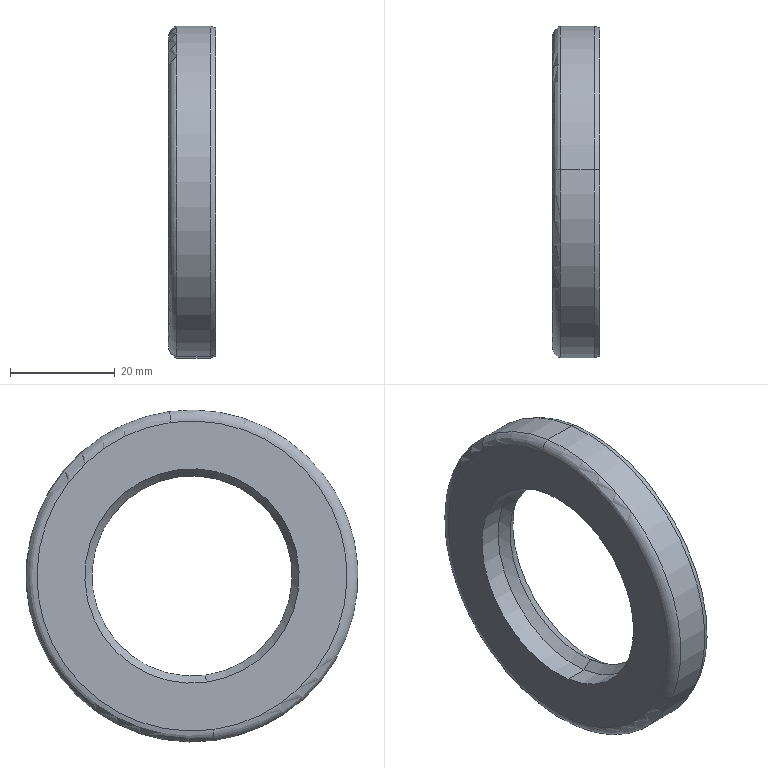Part | NX | features BREP 1 | 1 solid | 32 faces | box 9 x 63.5 x 63.5 mm | volume 6272 mm3 | torus 10 | cylinder 10 | cone 8 | plane 4 | commonest cylinder face diameters 45.17 x4 41 x2 61.3 x2 63.5 x2
STEP:
#1=CARTESIAN_POINT('',(-548.52,3.047,22.378));
#2=VERTEX_POINT('',#1);
#3=CARTESIAN_POINT('',(-548.52,-3.047,-22.378));
#4=VERTEX_POINT('',#3);
#5=CARTESIAN_POINT('',(-548.52,0.,0.));
#6=DIRECTION('',(-1.,0.,0.));
#7=DIRECTION('',(0.,0.1349,0.9909));
#8=AXIS2_PLACEMENT_3D('',#5,#6,#7);
#9=CIRCLE('',#8,22.585);
#10=EDGE_CURVE('',#2,#4,#9,.T.);
#11=ORIENTED_EDGE('',*,*,#10,.T.);
#12=CARTESIAN_POINT('',(-551.12,-3.047,-22.378));
#13=VERTEX_POINT('',#12);
#14=CARTESIAN_POINT('',(-549.82,-3.047,-22.378));
#15=DIRECTION('',(0.,0.9909,-0.1349));
#16=DIRECTION('',(0.,0.1349,0.9909));
#17=AXIS2_PLACEMENT_3D('',#14,#15,#16);
#18=CIRCLE('',#17,1.3);
#19=EDGE_CURVE('',#4,#13,#18,.T.);
#20=ORIENTED_EDGE('',*,*,#19,.T.);
#21=CARTESIAN_POINT('',(-551.12,3.047,22.378));
#22=VERTEX_POINT('',#21);
#23=CARTESIAN_POINT('',(-551.12,0.,0.));
#24=DIRECTION('',(1.,0.,0.));
#25=DIRECTION('',(0.,-0.1349,-0.9909));
#26=AXIS2_PLACEMENT_3D('',#23,#24,#25);
#27=CIRCLE('',#26,22.585);
#28=EDGE_CURVE('',#13,#22,#27,.T.);
#29=ORIENTED_EDGE('',*,*,#28,.T.);
#30=CARTESIAN_POINT('',(-549.82,3.047,22.378));
#31=DIRECTION('',(0.,-0.9909,0.1349));
#32=DIRECTION('',(0.,-0.1349,-0.9909));
#33=AXIS2_PLACEMENT_3D('',#30,#31,#32);
#34=CIRCLE('',#33,1.3);
#35=EDGE_CURVE('',#2,#22,#34,.T.);
#36=ORIENTED_EDGE('',*,*,#35,.F.);
#37=EDGE_LOOP('',(#11,#20,#29,#36));
#38=FACE_BOUND('',#37,.T.);
#39=CARTESIAN_POINT('',(-549.82,0.,0.));
#40=DIRECTION('',(-1.,0.,0.));
#41=DIRECTION('',(0.,-0.1349,-0.9909));
#42=AXIS2_PLACEMENT_3D('',#39,#40,#41);
#43=TOROIDAL_SURFACE('',#42,22.585,1.3);
#44=ADVANCED_FACE('',(#38),#43,.T.);
#45=CARTESIAN_POINT('',(-548.02,4.284,31.46));
#46=VERTEX_POINT('',#45);
#47=CARTESIAN_POINT('',(-548.02,-4.284,-31.46));
#48=VERTEX_POINT('',#47);
#49=CARTESIAN_POINT('',(-548.02,0.,0.));
#50=DIRECTION('',(-1.,0.,0.));
#51=DIRECTION('',(0.,0.1349,0.9909));
#52=AXIS2_PLACEMENT_3D('',#49,#50,#51);
#53=CIRCLE('',#52,31.75);
#54=EDGE_CURVE('',#46,#48,#53,.T.);
#55=ORIENTED_EDGE('',*,*,#54,.T.);
#56=CARTESIAN_POINT('',(-554.476,-4.284,-31.46));
#57=VERTEX_POINT('',#56);
#58=CARTESIAN_POINT('',(-556.022,-4.284,-31.46));
#59=DIRECTION('',(-1.,0.,0.));
#60=VECTOR('',#59,1000.);
#61=LINE('',#58,#60);
#62=EDGE_CURVE('',#48,#57,#61,.T.);
#63=ORIENTED_EDGE('',*,*,#62,.T.);
#64=CARTESIAN_POINT('',(-554.476,4.284,31.46));
#65=VERTEX_POINT('',#64);
#66=CARTESIAN_POINT('',(-554.476,0.,0.));
#67=DIRECTION('',(-1.,0.,0.));
#68=DIRECTION('',(0.,0.1349,0.9909));
#69=AXIS2_PLACEMENT_3D('',#66,#67,#68);
#70=CIRCLE('',#69,31.75);
#71=EDGE_CURVE('',#65,#57,#70,.T.);
#72=ORIENTED_EDGE('',*,*,#71,.F.);
#73=CARTESIAN_POINT('',(-556.022,4.284,31.46));
#74=DIRECTION('',(-1.,0.,0.));
#75=VECTOR('',#74,1000.);
#76=LINE('',#73,#75);
#77=EDGE_CURVE('',#46,#65,#76,.T.);
#78=ORIENTED_EDGE('',*,*,#77,.F.);
#79=EDGE_LOOP('',(#55,#63,#72,#78));
#80=FACE_BOUND('',#79,.T.);
#81=CARTESIAN_POINT('',(-556.022,0.,0.));
#82=DIRECTION('',(-1.,0.,0.));
#83=DIRECTION('',(0.,-0.1349,-0.9909));
#84=AXIS2_PLACEMENT_3D('',#81,#82,#83);
#85=CYLINDRICAL_SURFACE('',#84,31.75);
#86=ADVANCED_FACE('',(#80),#85,.T.);
#87=CARTESIAN_POINT('',(-547.02,4.235,31.099));
#88=VERTEX_POINT('',#87);
#89=CARTESIAN_POINT('',(-547.02,-4.235,-31.099));
#90=VERTEX_POINT('',#89);
#91=CARTESIAN_POINT('',(-547.02,0.,0.));
#92=DIRECTION('',(-1.,0.,0.));
#93=DIRECTION('',(0.,0.1349,0.9909));
#94=AXIS2_PLACEMENT_3D('',#91,#92,#93);
#95=CIRCLE('',#94,31.386);
#96=EDGE_CURVE('',#88,#90,#95,.T.);
#97=ORIENTED_EDGE('',*,*,#96,.T.);
#98=CARTESIAN_POINT('',(-547.02,-4.235,-31.099));
#99=DIRECTION('',(-0.9397,-0.04615,-0.3389));
#100=VECTOR('',#99,1000.);
#101=LINE('',#98,#100);
#102=EDGE_CURVE('',#90,#48,#101,.T.);
#103=ORIENTED_EDGE('',*,*,#102,.T.);
#104=ORIENTED_EDGE('',*,*,#54,.F.);
#105=CARTESIAN_POINT('',(-547.02,4.235,31.099));
#106=DIRECTION('',(-0.9397,0.04615,0.3389));
#107=VECTOR('',#106,1000.);
#108=LINE('',#105,#107);
#109=EDGE_CURVE('',#88,#46,#108,.T.);
#110=ORIENTED_EDGE('',*,*,#109,.F.);
#111=EDGE_LOOP('',(#97,#103,#104,#110));
#112=FACE_BOUND('',#111,.T.);
#113=CARTESIAN_POINT('',(-547.02,0.,0.));
#114=DIRECTION('',(-1.,0.,0.));
#115=DIRECTION('',(0.,-0.1349,-0.9909));
#116=AXIS2_PLACEMENT_3D('',#113,#114,#115);
#117=CONICAL_SURFACE('',#116,31.386,0.3491);
#118=ADVANCED_FACE('',(#112),#117,.T.);
#119=CARTESIAN_POINT('',(-547.02,-4.136,-30.37));
#120=VERTEX_POINT('',#119);
#121=CARTESIAN_POINT('',(-547.02,4.136,30.37));
#122=VERTEX_POINT('',#121);
#123=CARTESIAN_POINT('',(-547.02,0.,0.));
#124=DIRECTION('',(-1.,0.,0.));
#125=DIRECTION('',(0.,0.1349,0.9909));
#126=AXIS2_PLACEMENT_3D('',#123,#124,#125);
#127=CIRCLE('',#126,30.65);
#128=EDGE_CURVE('',#120,#122,#127,.T.);
#129=ORIENTED_EDGE('',*,*,#128,.F.);
#130=CARTESIAN_POINT('',(-553.82,-4.136,-30.37));
#131=VERTEX_POINT('',#130);
#132=CARTESIAN_POINT('',(-556.022,-4.136,-30.37));
#133=DIRECTION('',(-1.,0.,0.));
#134=VECTOR('',#133,1000.);
#135=LINE('',#132,#134);
#136=EDGE_CURVE('',#120,#131,#135,.T.);
#137=ORIENTED_EDGE('',*,*,#136,.T.);
#138=CARTESIAN_POINT('',(-553.82,4.136,30.37));
#139=VERTEX_POINT('',#138);
#140=CARTESIAN_POINT('',(-553.82,0.,0.));
#141=DIRECTION('',(-1.,0.,0.));
#142=DIRECTION('',(0.,0.1349,0.9909));
#143=AXIS2_PLACEMENT_3D('',#140,#141,#142);
#144=CIRCLE('',#143,30.65);
#145=EDGE_CURVE('',#131,#139,#144,.T.);
#146=ORIENTED_EDGE('',*,*,#145,.T.);
#147=CARTESIAN_POINT('',(-556.022,4.136,30.37));
#148=DIRECTION('',(-1.,0.,0.));
#149=VECTOR('',#148,1000.);
#150=LINE('',#147,#149);
#151=EDGE_CURVE('',#122,#139,#150,.T.);
#152=ORIENTED_EDGE('',*,*,#151,.F.);
#153=EDGE_LOOP('',(#129,#137,#146,#152));
#154=FACE_BOUND('',#153,.T.);
#155=CARTESIAN_POINT('',(-556.022,0.,0.));
#156=DIRECTION('',(-1.,0.,0.));
#157=DIRECTION('',(0.,-0.1349,-0.9909));
#158=AXIS2_PLACEMENT_3D('',#155,#156,#157);
#159=CYLINDRICAL_SURFACE('',#158,30.65);
#160=ADVANCED_FACE('',(#154),#159,.F.);
#161=ORIENTED_EDGE('',*,*,#145,.F.);
#162=CARTESIAN_POINT('',(-554.82,-4.001,-29.379));
#163=VERTEX_POINT('',#162);
#164=CARTESIAN_POINT('',(-553.82,-4.001,-29.379));
#165=DIRECTION('',(0.,0.9909,-0.1349));
#166=DIRECTION('',(0.,0.1349,0.9909));
#167=AXIS2_PLACEMENT_3D('',#164,#165,#166);
#168=CIRCLE('',#167,1.);
#169=EDGE_CURVE('',#131,#163,#168,.T.);
#170=ORIENTED_EDGE('',*,*,#169,.T.);
#171=CARTESIAN_POINT('',(-554.82,4.001,29.379));
#172=VERTEX_POINT('',#171);
#173=CARTESIAN_POINT('',(-554.82,0.,0.));
#174=DIRECTION('',(-1.,0.,0.));
#175=DIRECTION('',(0.,0.1349,0.9909));
#176=AXIS2_PLACEMENT_3D('',#173,#174,#175);
#177=CIRCLE('',#176,29.65);
#178=EDGE_CURVE('',#163,#172,#177,.T.);
#179=ORIENTED_EDGE('',*,*,#178,.T.);
#180=CARTESIAN_POINT('',(-553.82,4.001,29.379));
#181=DIRECTION('',(0.,-0.9909,0.1349));
#182=DIRECTION('',(0.,-0.1349,-0.9909));
#183=AXIS2_PLACEMENT_3D('',#180,#181,#182);
#184=CIRCLE('',#183,1.);
#185=EDGE_CURVE('',#139,#172,#184,.T.);
#186=ORIENTED_EDGE('',*,*,#185,.F.);
#187=EDGE_LOOP('',(#161,#170,#179,#186));
#188=FACE_BOUND('',#187,.T.);
#189=CARTESIAN_POINT('',(-553.82,0.,0.));
#190=DIRECTION('',(-1.,0.,0.));
#191=DIRECTION('',(0.,-0.1349,-0.9909));
#192=AXIS2_PLACEMENT_3D('',#189,#190,#191);
#193=TOROIDAL_SURFACE('',#192,29.65,1.);
#194=ADVANCED_FACE('',(#188),#193,.F.);
#195=ORIENTED_EDGE('',*,*,#71,.T.);
#196=CARTESIAN_POINT('',(-556.02,-4.001,-29.379));
#197=VERTEX_POINT('',#196);
#198=CARTESIAN_POINT('',(-553.82,-4.001,-29.379));
#199=DIRECTION('',(0.,0.9909,-0.1349));
#200=DIRECTION('',(0.,0.1349,0.9909));
#201=AXIS2_PLACEMENT_3D('',#198,#199,#200);
#202=CIRCLE('',#201,2.2);
#203=EDGE_CURVE('',#57,#197,#202,.T.);
#204=ORIENTED_EDGE('',*,*,#203,.T.);
#205=CARTESIAN_POINT('',(-556.02,4.001,29.379));
#206=VERTEX_POINT('',#205);
#207=CARTESIAN_POINT('',(-556.02,0.,0.));
#208=DIRECTION('',(-1.,0.,0.));
#209=DIRECTION('',(0.,0.1349,0.9909));
#210=AXIS2_PLACEMENT_3D('',#207,#208,#209);
#211=CIRCLE('',#210,29.65);
#212=EDGE_CURVE('',#206,#197,#211,.T.);
#213=ORIENTED_EDGE('',*,*,#212,.F.);
#214=CARTESIAN_POINT('',(-553.82,4.001,29.379));
#215=DIRECTION('',(0.,-0.9909,0.1349));
#216=DIRECTION('',(0.,-0.1349,-0.9909));
#217=AXIS2_PLACEMENT_3D('',#214,#215,#216);
#218=CIRCLE('',#217,2.2);
#219=EDGE_CURVE('',#65,#206,#218,.T.);
#220=ORIENTED_EDGE('',*,*,#219,.F.);
#221=EDGE_LOOP('',(#195,#204,#213,#220));
#222=FACE_BOUND('',#221,.T.);
#223=CARTESIAN_POINT('',(-553.82,0.,0.));
#224=DIRECTION('',(-1.,0.,0.));
#225=DIRECTION('',(0.,-0.1349,-0.9909));
#226=AXIS2_PLACEMENT_3D('',#223,#224,#225);
#227=TOROIDAL_SURFACE('',#226,29.65,2.2);
#228=ADVANCED_FACE('',(#222),#227,.T.);
#229=ORIENTED_EDGE('',*,*,#28,.F.);
#230=CARTESIAN_POINT('',(-554.,-3.047,-22.378));
#231=VERTEX_POINT('',#230);
#232=CARTESIAN_POINT('',(-556.022,-3.047,-22.378));
#233=DIRECTION('',(-1.,0.,0.));
#234=VECTOR('',#233,1000.);
#235=LINE('',#232,#234);
#236=EDGE_CURVE('',#13,#231,#235,.T.);
#237=ORIENTED_EDGE('',*,*,#236,.T.);
#238=CARTESIAN_POINT('',(-554.,3.047,22.378));
#239=VERTEX_POINT('',#238);
#240=CARTESIAN_POINT('',(-554.,0.,0.));
#241=DIRECTION('',(-1.,0.,0.));
#242=DIRECTION('',(0.,0.1349,0.9909));
#243=AXIS2_PLACEMENT_3D('',#240,#241,#242);
#244=CIRCLE('',#243,22.585);
#245=EDGE_CURVE('',#239,#231,#244,.T.);
#246=ORIENTED_EDGE('',*,*,#245,.F.);
#247=CARTESIAN_POINT('',(-556.022,3.047,22.378));
#248=DIRECTION('',(-1.,0.,0.));
#249=VECTOR('',#248,1000.);
#250=LINE('',#247,#249);
#251=EDGE_CURVE('',#22,#239,#250,.T.);
#252=ORIENTED_EDGE('',*,*,#251,.F.);
#253=EDGE_LOOP('',(#229,#237,#246,#252));
#254=FACE_BOUND('',#253,.T.);
#255=CARTESIAN_POINT('',(-556.022,0.,0.));
#256=DIRECTION('',(-1.,0.,0.));
#257=DIRECTION('',(0.,-0.1349,-0.9909));
#258=AXIS2_PLACEMENT_3D('',#255,#256,#257);
#259=CYLINDRICAL_SURFACE('',#258,22.585);
#260=ADVANCED_FACE('',(#254),#259,.T.);
#261=ORIENTED_EDGE('',*,*,#245,.T.);
#262=CARTESIAN_POINT('',(-554.82,-3.166,-23.247));
#263=VERTEX_POINT('',#262);
#264=CARTESIAN_POINT('',(-554.,-3.047,-22.378));
#265=DIRECTION('',(-0.6835,-0.09849,-0.7233));
#266=VECTOR('',#265,1000.);
#267=LINE('',#264,#266);
#268=EDGE_CURVE('',#231,#263,#267,.T.);
#269=ORIENTED_EDGE('',*,*,#268,.T.);
#270=CARTESIAN_POINT('',(-554.82,3.166,23.247));
#271=VERTEX_POINT('',#270);
#272=CARTESIAN_POINT('',(-554.82,0.,0.));
#273=DIRECTION('',(-1.,0.,0.));
#274=DIRECTION('',(0.,0.1349,0.9909));
#275=AXIS2_PLACEMENT_3D('',#272,#273,#274);
#276=CIRCLE('',#275,23.461);
#277=EDGE_CURVE('',#271,#263,#276,.T.);
#278=ORIENTED_EDGE('',*,*,#277,.F.);
#279=CARTESIAN_POINT('',(-554.,3.047,22.378));
#280=DIRECTION('',(-0.6835,0.09849,0.7233));
#281=VECTOR('',#280,1000.);
#282=LINE('',#279,#281);
#283=EDGE_CURVE('',#239,#271,#282,.T.);
#284=ORIENTED_EDGE('',*,*,#283,.F.);
#285=EDGE_LOOP('',(#261,#269,#278,#284));
#286=FACE_BOUND('',#285,.T.);
#287=CARTESIAN_POINT('',(-554.,0.,0.));
#288=DIRECTION('',(-1.,0.,0.));
#289=DIRECTION('',(0.,-0.1349,-0.9909));
#290=AXIS2_PLACEMENT_3D('',#287,#288,#289);
#291=CONICAL_SURFACE('',#290,22.585,0.8183);
#292=ADVANCED_FACE('',(#286),#291,.T.);
#293=CARTESIAN_POINT('',(-551.678,-2.766,-20.313));
#294=VERTEX_POINT('',#293);
#295=CARTESIAN_POINT('',(-551.678,2.766,20.313));
#296=VERTEX_POINT('',#295);
#297=CARTESIAN_POINT('',(-551.678,0.,0.));
#298=DIRECTION('',(-1.,0.,0.));
#299=DIRECTION('',(0.,0.1349,0.9909));
#300=AXIS2_PLACEMENT_3D('',#297,#298,#299);
#301=CIRCLE('',#300,20.5);
#302=EDGE_CURVE('',#294,#296,#301,.T.);
#303=ORIENTED_EDGE('',*,*,#302,.F.);
#304=CARTESIAN_POINT('',(-556.02,-2.766,-20.313));
#305=VERTEX_POINT('',#304);
#306=CARTESIAN_POINT('',(-556.022,-2.766,-20.313));
#307=DIRECTION('',(-1.,0.,0.));
#308=VECTOR('',#307,1000.);
#309=LINE('',#306,#308);
#310=EDGE_CURVE('',#294,#305,#309,.T.);
#311=ORIENTED_EDGE('',*,*,#310,.T.);
#312=CARTESIAN_POINT('',(-556.02,2.766,20.313));
#313=VERTEX_POINT('',#312);
#314=CARTESIAN_POINT('',(-556.02,0.,0.));
#315=DIRECTION('',(-1.,0.,0.));
#316=DIRECTION('',(0.,0.1349,0.9909));
#317=AXIS2_PLACEMENT_3D('',#314,#315,#316);
#318=CIRCLE('',#317,20.5);
#319=EDGE_CURVE('',#305,#313,#318,.T.);
#320=ORIENTED_EDGE('',*,*,#319,.T.);
#321=CARTESIAN_POINT('',(-556.022,2.766,20.313));
#322=DIRECTION('',(-1.,0.,0.));
#323=VECTOR('',#322,1000.);
#324=LINE('',#321,#323);
#325=EDGE_CURVE('',#296,#313,#324,.T.);
#326=ORIENTED_EDGE('',*,*,#325,.F.);
#327=EDGE_LOOP('',(#303,#311,#320,#326));
#328=FACE_BOUND('',#327,.T.);
#329=CARTESIAN_POINT('',(-556.022,0.,0.));
#330=DIRECTION('',(-1.,0.,0.));
#331=DIRECTION('',(0.,-0.1349,-0.9909));
#332=AXIS2_PLACEMENT_3D('',#329,#330,#331);
#333=CYLINDRICAL_SURFACE('',#332,20.5);
#334=ADVANCED_FACE('',(#328),#333,.F.);
#335=CARTESIAN_POINT('',(-549.82,-2.584,-18.975));
#336=VERTEX_POINT('',#335);
#337=CARTESIAN_POINT('',(-549.82,2.584,18.975));
#338=VERTEX_POINT('',#337);
#339=CARTESIAN_POINT('',(-549.82,0.,0.));
#340=DIRECTION('',(-1.,0.,0.));
#341=DIRECTION('',(0.,0.1349,0.9909));
#342=AXIS2_PLACEMENT_3D('',#339,#340,#341);
#343=CIRCLE('',#342,19.15);
#344=EDGE_CURVE('',#336,#338,#343,.T.);
#345=ORIENTED_EDGE('',*,*,#344,.F.);
#346=CARTESIAN_POINT('',(-551.678,-2.766,-20.313));
#347=DIRECTION('',(-0.809,-0.07931,-0.5824));
#348=VECTOR('',#347,1000.);
#349=LINE('',#346,#348);
#350=EDGE_CURVE('',#336,#294,#349,.T.);
#351=ORIENTED_EDGE('',*,*,#350,.T.);
#352=ORIENTED_EDGE('',*,*,#302,.T.);
#353=CARTESIAN_POINT('',(-551.678,2.766,20.313));
#354=DIRECTION('',(-0.809,0.07931,0.5824));
#355=VECTOR('',#354,1000.);
#356=LINE('',#353,#355);
#357=EDGE_CURVE('',#338,#296,#356,.T.);
#358=ORIENTED_EDGE('',*,*,#357,.F.);
#359=EDGE_LOOP('',(#345,#351,#352,#358));
#360=FACE_BOUND('',#359,.T.);
#361=CARTESIAN_POINT('',(-551.678,0.,0.));
#362=DIRECTION('',(-1.,0.,0.));
#363=DIRECTION('',(0.,-0.1349,-0.9909));
#364=AXIS2_PLACEMENT_3D('',#361,#362,#363);
#365=CONICAL_SURFACE('',#364,20.5,0.6283);
#366=ADVANCED_FACE('',(#360),#365,.F.);
#367=ORIENTED_EDGE('',*,*,#344,.T.);
#368=CARTESIAN_POINT('',(-547.62,2.777,20.397));
#369=VERTEX_POINT('',#368);
#370=CARTESIAN_POINT('',(-549.82,2.584,18.975));
#371=DIRECTION('',(0.8376,0.07371,0.5413));
#372=VECTOR('',#371,1000.);
#373=LINE('',#370,#372);
#374=EDGE_CURVE('',#369,#338,#373,.F.);
#375=ORIENTED_EDGE('',*,*,#374,.F.);
#376=CARTESIAN_POINT('',(-547.62,-2.777,-20.397));
#377=VERTEX_POINT('',#376);
#378=CARTESIAN_POINT('',(-547.62,0.,0.));
#379=DIRECTION('',(-1.,0.,0.));
#380=DIRECTION('',(0.,0.1349,0.9909));
#381=AXIS2_PLACEMENT_3D('',#378,#379,#380);
#382=CIRCLE('',#381,20.585);
#383=EDGE_CURVE('',#377,#369,#382,.T.);
#384=ORIENTED_EDGE('',*,*,#383,.F.);
#385=CARTESIAN_POINT('',(-549.82,-2.584,-18.975));
#386=DIRECTION('',(0.8376,-0.07371,-0.5413));
#387=VECTOR('',#386,1000.);
#388=LINE('',#385,#387);
#389=EDGE_CURVE('',#377,#336,#388,.F.);
#390=ORIENTED_EDGE('',*,*,#389,.T.);
#391=EDGE_LOOP('',(#367,#375,#384,#390));
#392=FACE_BOUND('',#391,.T.);
#393=CARTESIAN_POINT('',(-549.82,0.,0.));
#394=DIRECTION('',(1.,0.,0.));
#395=DIRECTION('',(0.,0.1349,0.9909));
#396=AXIS2_PLACEMENT_3D('',#393,#394,#395);
#397=CONICAL_SURFACE('',#396,19.15,0.578);
#398=ADVANCED_FACE('',(#392),#397,.F.);
#399=CARTESIAN_POINT('',(-547.62,3.047,22.378));
#400=VERTEX_POINT('',#399);
#401=CARTESIAN_POINT('',(-547.62,-3.047,-22.378));
#402=VERTEX_POINT('',#401);
#403=CARTESIAN_POINT('',(-547.62,0.,0.));
#404=DIRECTION('',(-1.,0.,0.));
#405=DIRECTION('',(0.,0.1349,0.9909));
#406=AXIS2_PLACEMENT_3D('',#403,#404,#405);
#407=CIRCLE('',#406,22.585);
#408=EDGE_CURVE('',#400,#402,#407,.T.);
#409=ORIENTED_EDGE('',*,*,#408,.T.);
#410=CARTESIAN_POINT('',(-556.022,-3.047,-22.378));
#411=DIRECTION('',(-1.,0.,0.));
#412=VECTOR('',#411,1000.);
#413=LINE('',#410,#412);
#414=EDGE_CURVE('',#402,#4,#413,.T.);
#415=ORIENTED_EDGE('',*,*,#414,.T.);
#416=ORIENTED_EDGE('',*,*,#10,.F.);
#417=CARTESIAN_POINT('',(-556.022,3.047,22.378));
#418=DIRECTION('',(-1.,0.,0.));
#419=VECTOR('',#418,1000.);
#420=LINE('',#417,#419);
#421=EDGE_CURVE('',#400,#2,#420,.T.);
#422=ORIENTED_EDGE('',*,*,#421,.F.);
#423=EDGE_LOOP('',(#409,#415,#416,#422));
#424=FACE_BOUND('',#423,.T.);
#425=CARTESIAN_POINT('',(-556.022,0.,0.));
#426=DIRECTION('',(-1.,0.,0.));
#427=DIRECTION('',(0.,-0.1349,-0.9909));
#428=AXIS2_PLACEMENT_3D('',#425,#426,#427);
#429=CYLINDRICAL_SURFACE('',#428,22.585);
#430=ADVANCED_FACE('',(#424),#429,.T.);
#431=ORIENTED_EDGE('',*,*,#414,.F.);
#432=CARTESIAN_POINT('',(-547.62,0.,0.));
#433=DIRECTION('',(-1.,0.,0.));
#434=DIRECTION('',(0.,0.1349,0.9909));
#435=AXIS2_PLACEMENT_3D('',#432,#433,#434);
#436=CIRCLE('',#435,22.585);
#437=EDGE_CURVE('',#402,#400,#436,.T.);
#438=ORIENTED_EDGE('',*,*,#437,.T.);
#439=ORIENTED_EDGE('',*,*,#421,.T.);
#440=CARTESIAN_POINT('',(-548.52,0.,0.));
#441=DIRECTION('',(-1.,0.,0.));
#442=DIRECTION('',(0.,0.1349,0.9909));
#443=AXIS2_PLACEMENT_3D('',#440,#441,#442);
#444=CIRCLE('',#443,22.585);
#445=EDGE_CURVE('',#4,#2,#444,.T.);
#446=ORIENTED_EDGE('',*,*,#445,.F.);
#447=EDGE_LOOP('',(#431,#438,#439,#446));
#448=FACE_BOUND('',#447,.T.);
#449=CARTESIAN_POINT('',(-556.022,0.,0.));
#450=DIRECTION('',(-1.,0.,0.));
#451=DIRECTION('',(0.,-0.1349,-0.9909));
#452=AXIS2_PLACEMENT_3D('',#449,#450,#451);
#453=CYLINDRICAL_SURFACE('',#452,22.585);
#454=ADVANCED_FACE('',(#448),#453,.T.);
#455=ORIENTED_EDGE('',*,*,#408,.F.);
#456=ORIENTED_EDGE('',*,*,#437,.F.);
#457=EDGE_LOOP('',(#455,#456));
#458=FACE_BOUND('',#457,.T.);
#459=ORIENTED_EDGE('',*,*,#383,.T.);
#460=CARTESIAN_POINT('',(-547.62,0.,0.));
#461=DIRECTION('',(-1.,0.,0.));
#462=DIRECTION('',(0.,0.1349,0.9909));
#463=AXIS2_PLACEMENT_3D('',#460,#461,#462);
#464=CIRCLE('',#463,20.585);
#465=EDGE_CURVE('',#369,#377,#464,.T.);
#466=ORIENTED_EDGE('',*,*,#465,.T.);
#467=EDGE_LOOP('',(#459,#466));
#468=FACE_BOUND('',#467,.T.);
#469=CARTESIAN_POINT('',(-547.62,20.397,-2.777));
#470=DIRECTION('',(-1.,0.,0.));
#471=DIRECTION('',(0.,-0.1349,-0.9909));
#472=AXIS2_PLACEMENT_3D('',#469,#470,#471);
#473=PLANE('',#472);
#474=ADVANCED_FACE('',(#458,#468),#473,.F.);
#475=ORIENTED_EDGE('',*,*,#374,.T.);
#476=CARTESIAN_POINT('',(-549.82,0.,0.));
#477=DIRECTION('',(-1.,0.,0.));
#478=DIRECTION('',(0.,0.1349,0.9909));
#479=AXIS2_PLACEMENT_3D('',#476,#477,#478);
#480=CIRCLE('',#479,19.15);
#481=EDGE_CURVE('',#338,#336,#480,.T.);
#482=ORIENTED_EDGE('',*,*,#481,.T.);
#483=ORIENTED_EDGE('',*,*,#389,.F.);
#484=ORIENTED_EDGE('',*,*,#465,.F.);
#485=EDGE_LOOP('',(#475,#482,#483,#484));
#486=FACE_BOUND('',#485,.T.);
#487=CARTESIAN_POINT('',(-549.82,0.,0.));
#488=DIRECTION('',(1.,0.,0.));
#489=DIRECTION('',(0.,0.1349,0.9909));
#490=AXIS2_PLACEMENT_3D('',#487,#488,#489);
#491=CONICAL_SURFACE('',#490,19.15,0.578);
#492=ADVANCED_FACE('',(#486),#491,.F.);
#493=ORIENTED_EDGE('',*,*,#350,.F.);
#494=ORIENTED_EDGE('',*,*,#481,.F.);
#495=ORIENTED_EDGE('',*,*,#357,.T.);
#496=CARTESIAN_POINT('',(-551.678,0.,0.));
#497=DIRECTION('',(-1.,0.,0.));
#498=DIRECTION('',(0.,0.1349,0.9909));
#499=AXIS2_PLACEMENT_3D('',#496,#497,#498);
#500=CIRCLE('',#499,20.5);
#501=EDGE_CURVE('',#296,#294,#500,.T.);
#502=ORIENTED_EDGE('',*,*,#501,.T.);
#503=EDGE_LOOP('',(#493,#494,#495,#502));
#504=FACE_BOUND('',#503,.T.);
#505=CARTESIAN_POINT('',(-551.678,0.,0.));
#506=DIRECTION('',(-1.,0.,0.));
#507=DIRECTION('',(0.,-0.1349,-0.9909));
#508=AXIS2_PLACEMENT_3D('',#505,#506,#507);
#509=CONICAL_SURFACE('',#508,20.5,0.6283);
#510=ADVANCED_FACE('',(#504),#509,.F.);
#511=ORIENTED_EDGE('',*,*,#310,.F.);
#512=ORIENTED_EDGE('',*,*,#501,.F.);
#513=ORIENTED_EDGE('',*,*,#325,.T.);
#514=CARTESIAN_POINT('',(-556.02,0.,0.));
#515=DIRECTION('',(-1.,0.,0.));
#516=DIRECTION('',(0.,0.1349,0.9909));
#517=AXIS2_PLACEMENT_3D('',#514,#515,#516);
#518=CIRCLE('',#517,20.5);
#519=EDGE_CURVE('',#313,#305,#518,.T.);
#520=ORIENTED_EDGE('',*,*,#519,.T.);
#521=EDGE_LOOP('',(#511,#512,#513,#520));
#522=FACE_BOUND('',#521,.T.);
#523=CARTESIAN_POINT('',(-556.022,0.,0.));
#524=DIRECTION('',(-1.,0.,0.));
#525=DIRECTION('',(0.,-0.1349,-0.9909));
#526=AXIS2_PLACEMENT_3D('',#523,#524,#525);
#527=CYLINDRICAL_SURFACE('',#526,20.5);
#528=ADVANCED_FACE('',(#522),#527,.F.);
#529=ORIENTED_EDGE('',*,*,#519,.F.);
#530=ORIENTED_EDGE('',*,*,#319,.F.);
#531=EDGE_LOOP('',(#529,#530));
#532=FACE_BOUND('',#531,.T.);
#533=ORIENTED_EDGE('',*,*,#212,.T.);
#534=CARTESIAN_POINT('',(-556.02,0.,0.));
#535=DIRECTION('',(-1.,0.,0.));
#536=DIRECTION('',(0.,0.1349,0.9909));
#537=AXIS2_PLACEMENT_3D('',#534,#535,#536);
#538=CIRCLE('',#537,29.65);
#539=EDGE_CURVE('',#197,#206,#538,.T.);
#540=ORIENTED_EDGE('',*,*,#539,.T.);
#541=EDGE_LOOP('',(#533,#540));
#542=FACE_BOUND('',#541,.T.);
#543=CARTESIAN_POINT('',(-556.02,22.827,-3.108));
#544=DIRECTION('',(1.,0.,0.));
#545=DIRECTION('',(0.,0.1349,0.9909));
#546=AXIS2_PLACEMENT_3D('',#543,#544,#545);
#547=PLANE('',#546);
#548=ADVANCED_FACE('',(#532,#542),#547,.F.);
#549=ORIENTED_EDGE('',*,*,#268,.F.);
#550=CARTESIAN_POINT('',(-554.,0.,0.));
#551=DIRECTION('',(-1.,0.,0.));
#552=DIRECTION('',(0.,0.1349,0.9909));
#553=AXIS2_PLACEMENT_3D('',#550,#551,#552);
#554=CIRCLE('',#553,22.585);
#555=EDGE_CURVE('',#231,#239,#554,.T.);
#556=ORIENTED_EDGE('',*,*,#555,.T.);
#557=ORIENTED_EDGE('',*,*,#283,.T.);
#558=CARTESIAN_POINT('',(-554.82,0.,0.));
#559=DIRECTION('',(-1.,0.,0.));
#560=DIRECTION('',(0.,0.1349,0.9909));
#561=AXIS2_PLACEMENT_3D('',#558,#559,#560);
#562=CIRCLE('',#561,23.461);
#563=EDGE_CURVE('',#263,#271,#562,.T.);
#564=ORIENTED_EDGE('',*,*,#563,.F.);
#565=EDGE_LOOP('',(#549,#556,#557,#564));
#566=FACE_BOUND('',#565,.T.);
#567=CARTESIAN_POINT('',(-554.,0.,0.));
#568=DIRECTION('',(-1.,0.,0.));
#569=DIRECTION('',(0.,-0.1349,-0.9909));
#570=AXIS2_PLACEMENT_3D('',#567,#568,#569);
#571=CONICAL_SURFACE('',#570,22.585,0.8183);
#572=ADVANCED_FACE('',(#566),#571,.T.);
#573=ORIENTED_EDGE('',*,*,#236,.F.);
#574=CARTESIAN_POINT('',(-551.12,0.,0.));
#575=DIRECTION('',(1.,0.,0.));
#576=DIRECTION('',(0.,-0.1349,-0.9909));
#577=AXIS2_PLACEMENT_3D('',#574,#575,#576);
#578=CIRCLE('',#577,22.585);
#579=EDGE_CURVE('',#22,#13,#578,.T.);
#580=ORIENTED_EDGE('',*,*,#579,.F.);
#581=ORIENTED_EDGE('',*,*,#251,.T.);
#582=ORIENTED_EDGE('',*,*,#555,.F.);
#583=EDGE_LOOP('',(#573,#580,#581,#582));
#584=FACE_BOUND('',#583,.T.);
#585=CARTESIAN_POINT('',(-556.022,0.,0.));
#586=DIRECTION('',(-1.,0.,0.));
#587=DIRECTION('',(0.,-0.1349,-0.9909));
#588=AXIS2_PLACEMENT_3D('',#585,#586,#587);
#589=CYLINDRICAL_SURFACE('',#588,22.585);
#590=ADVANCED_FACE('',(#584),#589,.T.);
#591=ORIENTED_EDGE('',*,*,#203,.F.);
#592=CARTESIAN_POINT('',(-554.476,0.,0.));
#593=DIRECTION('',(-1.,0.,0.));
#594=DIRECTION('',(0.,0.1349,0.9909));
#595=AXIS2_PLACEMENT_3D('',#592,#593,#594);
#596=CIRCLE('',#595,31.75);
#597=EDGE_CURVE('',#57,#65,#596,.T.);
#598=ORIENTED_EDGE('',*,*,#597,.T.);
#599=ORIENTED_EDGE('',*,*,#219,.T.);
#600=ORIENTED_EDGE('',*,*,#539,.F.);
#601=EDGE_LOOP('',(#591,#598,#599,#600));
#602=FACE_BOUND('',#601,.T.);
#603=CARTESIAN_POINT('',(-553.82,0.,0.));
#604=DIRECTION('',(-1.,0.,0.));
#605=DIRECTION('',(0.,-0.1349,-0.9909));
#606=AXIS2_PLACEMENT_3D('',#603,#604,#605);
#607=TOROIDAL_SURFACE('',#606,29.65,2.2);
#608=ADVANCED_FACE('',(#602),#607,.T.);
#609=ORIENTED_EDGE('',*,*,#277,.T.);
#610=ORIENTED_EDGE('',*,*,#563,.T.);
#611=EDGE_LOOP('',(#609,#610));
#612=FACE_BOUND('',#611,.T.);
#613=CARTESIAN_POINT('',(-554.82,0.,0.));
#614=DIRECTION('',(-1.,0.,0.));
#615=DIRECTION('',(0.,0.1349,0.9909));
#616=AXIS2_PLACEMENT_3D('',#613,#614,#615);
#617=CIRCLE('',#616,29.65);
#618=EDGE_CURVE('',#172,#163,#617,.T.);
#619=ORIENTED_EDGE('',*,*,#618,.F.);
#620=ORIENTED_EDGE('',*,*,#178,.F.);
#621=EDGE_LOOP('',(#619,#620));
#622=FACE_BOUND('',#621,.T.);
#623=CARTESIAN_POINT('',(-554.82,22.827,-3.108));
#624=DIRECTION('',(-1.,0.,0.));
#625=DIRECTION('',(0.,-0.1349,-0.9909));
#626=AXIS2_PLACEMENT_3D('',#623,#624,#625);
#627=PLANE('',#626);
#628=ADVANCED_FACE('',(#612,#622),#627,.F.);
#629=ORIENTED_EDGE('',*,*,#169,.F.);
#630=CARTESIAN_POINT('',(-553.82,0.,0.));
#631=DIRECTION('',(-1.,0.,0.));
#632=DIRECTION('',(0.,0.1349,0.9909));
#633=AXIS2_PLACEMENT_3D('',#630,#631,#632);
#634=CIRCLE('',#633,30.65);
#635=EDGE_CURVE('',#139,#131,#634,.T.);
#636=ORIENTED_EDGE('',*,*,#635,.F.);
#637=ORIENTED_EDGE('',*,*,#185,.T.);
#638=ORIENTED_EDGE('',*,*,#618,.T.);
#639=EDGE_LOOP('',(#629,#636,#637,#638));
#640=FACE_BOUND('',#639,.T.);
#641=CARTESIAN_POINT('',(-553.82,0.,0.));
#642=DIRECTION('',(-1.,0.,0.));
#643=DIRECTION('',(0.,-0.1349,-0.9909));
#644=AXIS2_PLACEMENT_3D('',#641,#642,#643);
#645=TOROIDAL_SURFACE('',#644,29.65,1.);
#646=ADVANCED_FACE('',(#640),#645,.F.);
#647=ORIENTED_EDGE('',*,*,#136,.F.);
#648=CARTESIAN_POINT('',(-547.02,0.,0.));
#649=DIRECTION('',(-1.,0.,0.));
#650=DIRECTION('',(0.,0.1349,0.9909));
#651=AXIS2_PLACEMENT_3D('',#648,#649,#650);
#652=CIRCLE('',#651,30.65);
#653=EDGE_CURVE('',#122,#120,#652,.T.);
#654=ORIENTED_EDGE('',*,*,#653,.F.);
#655=ORIENTED_EDGE('',*,*,#151,.T.);
#656=ORIENTED_EDGE('',*,*,#635,.T.);
#657=EDGE_LOOP('',(#647,#654,#655,#656));
#658=FACE_BOUND('',#657,.T.);
#659=CARTESIAN_POINT('',(-556.022,0.,0.));
#660=DIRECTION('',(-1.,0.,0.));
#661=DIRECTION('',(0.,-0.1349,-0.9909));
#662=AXIS2_PLACEMENT_3D('',#659,#660,#661);
#663=CYLINDRICAL_SURFACE('',#662,30.65);
#664=ADVANCED_FACE('',(#658),#663,.F.);
#665=ORIENTED_EDGE('',*,*,#96,.F.);
#666=CARTESIAN_POINT('',(-547.02,0.,0.));
#667=DIRECTION('',(-1.,0.,0.));
#668=DIRECTION('',(0.,0.1349,0.9909));
#669=AXIS2_PLACEMENT_3D('',#666,#667,#668);
#670=CIRCLE('',#669,31.386);
#671=EDGE_CURVE('',#90,#88,#670,.T.);
#672=ORIENTED_EDGE('',*,*,#671,.F.);
#673=EDGE_LOOP('',(#665,#672));
#674=FACE_BOUND('',#673,.T.);
#675=ORIENTED_EDGE('',*,*,#653,.T.);
#676=ORIENTED_EDGE('',*,*,#128,.T.);
#677=EDGE_LOOP('',(#675,#676));
#678=FACE_BOUND('',#677,.T.);
#679=CARTESIAN_POINT('',(-547.02,30.37,-4.136));
#680=DIRECTION('',(-1.,0.,0.));
#681=DIRECTION('',(0.,-0.1349,-0.9909));
#682=AXIS2_PLACEMENT_3D('',#679,#680,#681);
#683=PLANE('',#682);
#684=ADVANCED_FACE('',(#674,#678),#683,.F.);
#685=ORIENTED_EDGE('',*,*,#102,.F.);
#686=ORIENTED_EDGE('',*,*,#671,.T.);
#687=ORIENTED_EDGE('',*,*,#109,.T.);
#688=CARTESIAN_POINT('',(-548.02,0.,0.));
#689=DIRECTION('',(-1.,0.,0.));
#690=DIRECTION('',(0.,0.1349,0.9909));
#691=AXIS2_PLACEMENT_3D('',#688,#689,#690);
#692=CIRCLE('',#691,31.75);
#693=EDGE_CURVE('',#48,#46,#692,.T.);
#694=ORIENTED_EDGE('',*,*,#693,.F.);
#695=EDGE_LOOP('',(#685,#686,#687,#694));
#696=FACE_BOUND('',#695,.T.);
#697=CARTESIAN_POINT('',(-547.02,0.,0.));
#698=DIRECTION('',(-1.,0.,0.));
#699=DIRECTION('',(0.,-0.1349,-0.9909));
#700=AXIS2_PLACEMENT_3D('',#697,#698,#699);
#701=CONICAL_SURFACE('',#700,31.386,0.3491);
#702=ADVANCED_FACE('',(#696),#701,.T.);
#703=ORIENTED_EDGE('',*,*,#62,.F.);
#704=ORIENTED_EDGE('',*,*,#693,.T.);
#705=ORIENTED_EDGE('',*,*,#77,.T.);
#706=ORIENTED_EDGE('',*,*,#597,.F.);
#707=EDGE_LOOP('',(#703,#704,#705,#706));
#708=FACE_BOUND('',#707,.T.);
#709=CARTESIAN_POINT('',(-556.022,0.,0.));
#710=DIRECTION('',(-1.,0.,0.));
#711=DIRECTION('',(0.,-0.1349,-0.9909));
#712=AXIS2_PLACEMENT_3D('',#709,#710,#711);
#713=CYLINDRICAL_SURFACE('',#712,31.75);
#714=ADVANCED_FACE('',(#708),#713,.T.);
#715=ORIENTED_EDGE('',*,*,#19,.F.);
#716=ORIENTED_EDGE('',*,*,#445,.T.);
#717=ORIENTED_EDGE('',*,*,#35,.T.);
#718=ORIENTED_EDGE('',*,*,#579,.T.);
#719=EDGE_LOOP('',(#715,#716,#717,#718));
#720=FACE_BOUND('',#719,.T.);
#721=CARTESIAN_POINT('',(-549.82,0.,0.));
#722=DIRECTION('',(-1.,0.,0.));
#723=DIRECTION('',(0.,-0.1349,-0.9909));
#724=AXIS2_PLACEMENT_3D('',#721,#722,#723);
#725=TOROIDAL_SURFACE('',#724,22.585,1.3);
#726=ADVANCED_FACE('',(#720),#725,.T.);
#727=CLOSED_SHELL('',(#44,#86,#118,#160,#194,#228,#260,#292,#334,#366,#398,#430,#454,#474,#492,#510,#528,#548,#572,#590,#608,#628,#646,#664,#684,#702,#714,#726));
#728=CARTESIAN_POINT('',(-549.82,-2.943,-21.616));
#729=VERTEX_POINT('',#728);
#730=CARTESIAN_POINT('',(-549.82,2.943,21.616));
#731=VERTEX_POINT('',#730);
#732=CARTESIAN_POINT('',(-549.82,0.,0.));
#733=DIRECTION('',(-1.,0.,0.));
#734=DIRECTION('',(0.,0.,1.));
#735=AXIS2_PLACEMENT_3D('',#732,#733,#734);
#736=CIRCLE('',#735,21.815);
#737=EDGE_CURVE('',#729,#731,#736,.F.);
#738=ORIENTED_EDGE('',*,*,#737,.F.);
#739=CARTESIAN_POINT('',(-549.82,-3.151,-23.141));
#740=VERTEX_POINT('',#739);
#741=CARTESIAN_POINT('',(-549.82,-3.047,-22.378));
#742=DIRECTION('',(0.,0.9909,-0.1349));
#743=DIRECTION('',(0.,0.1349,0.9909));
#744=AXIS2_PLACEMENT_3D('',#741,#742,#743);
#745=CIRCLE('',#744,0.77);
#746=EDGE_CURVE('',#729,#740,#745,.T.);
#747=ORIENTED_EDGE('',*,*,#746,.T.);
#748=CARTESIAN_POINT('',(-549.82,3.151,23.141));
#749=VERTEX_POINT('',#748);
#750=CARTESIAN_POINT('',(-549.82,0.,0.));
#751=DIRECTION('',(-1.,0.,0.));
#752=DIRECTION('',(0.,0.,1.));
#753=AXIS2_PLACEMENT_3D('',#750,#751,#752);
#754=CIRCLE('',#753,23.355);
#755=EDGE_CURVE('',#740,#749,#754,.F.);
#756=ORIENTED_EDGE('',*,*,#755,.T.);
#757=CARTESIAN_POINT('',(-549.82,3.047,22.378));
#758=DIRECTION('',(0.,-0.9909,0.1349));
#759=DIRECTION('',(0.,-0.1349,-0.9909));
#760=AXIS2_PLACEMENT_3D('',#757,#758,#759);
#761=CIRCLE('',#760,0.77);
#762=EDGE_CURVE('',#731,#749,#761,.T.);
#763=ORIENTED_EDGE('',*,*,#762,.F.);
#764=EDGE_LOOP('',(#738,#747,#756,#763));
#765=FACE_BOUND('',#764,.T.);
#766=CARTESIAN_POINT('',(-549.82,0.,0.));
#767=DIRECTION('',(-1.,0.,0.));
#768=DIRECTION('',(0.,-0.1349,-0.9909));
#769=AXIS2_PLACEMENT_3D('',#766,#767,#768);
#770=TOROIDAL_SURFACE('',#769,22.585,0.77);
#771=ADVANCED_FACE('',(#765),#770,.T.);
#772=CARTESIAN_POINT('',(-549.82,0.,0.));
#773=DIRECTION('',(-1.,0.,0.));
#774=DIRECTION('',(0.,0.,1.));
#775=AXIS2_PLACEMENT_3D('',#772,#773,#774);
#776=CIRCLE('',#775,21.815);
#777=EDGE_CURVE('',#731,#729,#776,.F.);
#778=ORIENTED_EDGE('',*,*,#777,.F.);
#779=ORIENTED_EDGE('',*,*,#762,.T.);
#780=CARTESIAN_POINT('',(-549.82,0.,0.));
#781=DIRECTION('',(-1.,0.,0.));
#782=DIRECTION('',(0.,0.,1.));
#783=AXIS2_PLACEMENT_3D('',#780,#781,#782);
#784=CIRCLE('',#783,23.355);
#785=EDGE_CURVE('',#749,#740,#784,.F.);
#786=ORIENTED_EDGE('',*,*,#785,.T.);
#787=ORIENTED_EDGE('',*,*,#746,.F.);
#788=EDGE_LOOP('',(#778,#779,#786,#787));
#789=FACE_BOUND('',#788,.T.);
#790=CARTESIAN_POINT('',(-549.82,0.,0.));
#791=DIRECTION('',(-1.,0.,0.));
#792=DIRECTION('',(0.,-0.1349,-0.9909));
#793=AXIS2_PLACEMENT_3D('',#790,#791,#792);
#794=TOROIDAL_SURFACE('',#793,22.585,0.77);
#795=ADVANCED_FACE('',(#789),#794,.T.);
#796=CARTESIAN_POINT('',(-549.82,3.047,22.378));
#797=DIRECTION('',(0.,-0.9909,0.1349));
#798=DIRECTION('',(0.,-0.1349,-0.9909));
#799=AXIS2_PLACEMENT_3D('',#796,#797,#798);
#800=CIRCLE('',#799,0.77);
#801=EDGE_CURVE('',#731,#749,#800,.F.);
#802=ORIENTED_EDGE('',*,*,#801,.F.);
#803=ORIENTED_EDGE('',*,*,#777,.T.);
#804=CARTESIAN_POINT('',(-549.82,-3.047,-22.378));
#805=DIRECTION('',(0.,0.9909,-0.1349));
#806=DIRECTION('',(0.,0.1349,0.9909));
#807=AXIS2_PLACEMENT_3D('',#804,#805,#806);
#808=CIRCLE('',#807,0.77);
#809=EDGE_CURVE('',#729,#740,#808,.F.);
#810=ORIENTED_EDGE('',*,*,#809,.T.);
#811=ORIENTED_EDGE('',*,*,#785,.F.);
#812=EDGE_LOOP('',(#802,#803,#810,#811));
#813=FACE_BOUND('',#812,.T.);
#814=CARTESIAN_POINT('',(-549.82,0.,0.));
#815=DIRECTION('',(-1.,0.,0.));
#816=DIRECTION('',(0.,-0.1349,-0.9909));
#817=AXIS2_PLACEMENT_3D('',#814,#815,#816);
#818=TOROIDAL_SURFACE('',#817,22.585,0.77);
#819=ADVANCED_FACE('',(#813),#818,.T.);
#820=ORIENTED_EDGE('',*,*,#809,.F.);
#821=ORIENTED_EDGE('',*,*,#737,.T.);
#822=ORIENTED_EDGE('',*,*,#801,.T.);
#823=ORIENTED_EDGE('',*,*,#755,.F.);
#824=EDGE_LOOP('',(#820,#821,#822,#823));
#825=FACE_BOUND('',#824,.T.);
#826=CARTESIAN_POINT('',(-549.82,0.,0.));
#827=DIRECTION('',(-1.,0.,0.));
#828=DIRECTION('',(0.,-0.1349,-0.9909));
#829=AXIS2_PLACEMENT_3D('',#826,#827,#828);
#830=TOROIDAL_SURFACE('',#829,22.585,0.77);
#831=ADVANCED_FACE('',(#825),#830,.T.);
#832=CLOSED_SHELL('',(#771,#795,#819,#831));
#833=ORIENTED_CLOSED_SHELL('',*,#832,.F.);
#834=BREP_WITH_VOIDS('',#727,(#833));
#835=(LENGTH_UNIT()NAMED_UNIT(*)SI_UNIT(.MILLI.,.METRE.));
#836=UNCERTAINTY_MEASURE_WITH_UNIT(LENGTH_MEASURE(0.00001),#835,'','');
#837=(NAMED_UNIT(*)PLANE_ANGLE_UNIT()SI_UNIT($,.RADIAN.));
#838=(NAMED_UNIT(*)SI_UNIT($,.STERADIAN.)SOLID_ANGLE_UNIT());
#839=(GEOMETRIC_REPRESENTATION_CONTEXT(3)GLOBAL_UNCERTAINTY_ASSIGNED_CONTEXT((#836))GLOBAL_UNIT_ASSIGNED_CONTEXT((#835,#837,#838))REPRESENTATION_CONTEXT('',''));
#840=ADVANCED_BREP_SHAPE_REPRESENTATION('',(#834),#839);